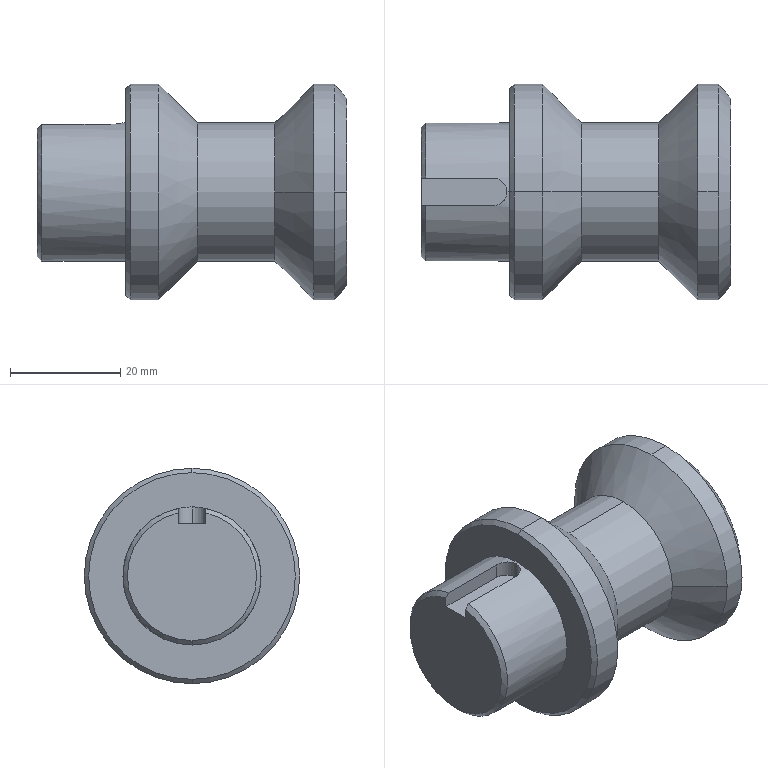Part | SolidWorks | features BaseBody 1 | 1 solid | 28 faces | box 56 x 39 x 39 mm | volume 37628 mm3 | cylinder 12 | cone 10 | plane 6 | commonest cylinder face diameters 25 x4 39 x4 5 x2 34 x2
STEP:
#1=CARTESIAN_POINT('',(61.076,0.,-17.));
#2=VERTEX_POINT('',#1);
#3=CARTESIAN_POINT('',(61.076,-17.,0.));
#4=VERTEX_POINT('',#3);
#5=CARTESIAN_POINT('',(61.076,0.,0.));
#6=DIRECTION('',(-1.,0.,0.));
#7=DIRECTION('',(0.,0.,1.));
#8=AXIS2_PLACEMENT_3D('',#5,#6,#7);
#9=CIRCLE('',#8,17.);
#10=EDGE_CURVE('',#2,#4,#9,.T.);
#11=ORIENTED_EDGE('',*,*,#10,.F.);
#12=CARTESIAN_POINT('',(58.576,0.,-17.));
#13=VERTEX_POINT('',#12);
#14=CARTESIAN_POINT('',(0.,0.,-17.));
#15=DIRECTION('',(-1.,0.,0.));
#16=VECTOR('',#15,1000.);
#17=LINE('',#14,#16);
#18=EDGE_CURVE('',#2,#13,#17,.T.);
#19=ORIENTED_EDGE('',*,*,#18,.T.);
#20=CARTESIAN_POINT('',(58.576,0.,17.));
#21=VERTEX_POINT('',#20);
#22=CARTESIAN_POINT('',(58.576,0.,0.));
#23=DIRECTION('',(1.,0.,0.));
#24=DIRECTION('',(0.,0.,1.));
#25=AXIS2_PLACEMENT_3D('',#22,#23,#24);
#26=CIRCLE('',#25,17.);
#27=EDGE_CURVE('',#21,#13,#26,.T.);
#28=ORIENTED_EDGE('',*,*,#27,.F.);
#29=CARTESIAN_POINT('',(61.076,0.,17.));
#30=VERTEX_POINT('',#29);
#31=CARTESIAN_POINT('',(0.,0.,17.));
#32=DIRECTION('',(-1.,0.,0.));
#33=VECTOR('',#32,1000.);
#34=LINE('',#31,#33);
#35=EDGE_CURVE('',#30,#21,#34,.T.);
#36=ORIENTED_EDGE('',*,*,#35,.F.);
#37=CARTESIAN_POINT('',(61.076,0.,0.));
#38=DIRECTION('',(-1.,0.,0.));
#39=DIRECTION('',(0.,0.,1.));
#40=AXIS2_PLACEMENT_3D('',#37,#38,#39);
#41=CIRCLE('',#40,17.);
#42=EDGE_CURVE('',#4,#30,#41,.T.);
#43=ORIENTED_EDGE('',*,*,#42,.F.);
#44=EDGE_LOOP('',(#11,#19,#28,#36,#43));
#45=FACE_OUTER_BOUND('',#44,.T.);
#46=CARTESIAN_POINT('',(0.,0.,0.));
#47=DIRECTION('',(-1.,0.,0.));
#48=DIRECTION('',(0.,0.,1.));
#49=AXIS2_PLACEMENT_3D('',#46,#47,#48);
#50=CYLINDRICAL_SURFACE('',#49,17.);
#51=ADVANCED_FACE('',(#45),#50,.F.);
#52=ORIENTED_EDGE('',*,*,#42,.T.);
#53=CARTESIAN_POINT('',(61.076,17.,0.));
#54=VERTEX_POINT('',#53);
#55=CARTESIAN_POINT('',(61.076,0.,0.));
#56=DIRECTION('',(-1.,0.,0.));
#57=DIRECTION('',(0.,0.,1.));
#58=AXIS2_PLACEMENT_3D('',#55,#56,#57);
#59=CIRCLE('',#58,17.);
#60=EDGE_CURVE('',#30,#54,#59,.T.);
#61=ORIENTED_EDGE('',*,*,#60,.T.);
#62=CARTESIAN_POINT('',(58.876,19.5,0.));
#63=VERTEX_POINT('',#62);
#64=CARTESIAN_POINT('',(58.876,19.5,0.));
#65=DIRECTION('',(-0.6606,0.7507,0.));
#66=VECTOR('',#65,1000.);
#67=LINE('',#64,#66);
#68=EDGE_CURVE('',#54,#63,#67,.T.);
#69=ORIENTED_EDGE('',*,*,#68,.T.);
#70=CARTESIAN_POINT('',(58.876,0.,19.5));
#71=VERTEX_POINT('',#70);
#72=CARTESIAN_POINT('',(58.876,0.,0.));
#73=DIRECTION('',(1.,0.,0.));
#74=DIRECTION('',(0.,0.,-1.));
#75=AXIS2_PLACEMENT_3D('',#72,#73,#74);
#76=CIRCLE('',#75,19.5);
#77=EDGE_CURVE('',#63,#71,#76,.T.);
#78=ORIENTED_EDGE('',*,*,#77,.T.);
#79=CARTESIAN_POINT('',(58.876,-19.5,0.));
#80=VERTEX_POINT('',#79);
#81=CARTESIAN_POINT('',(58.876,0.,0.));
#82=DIRECTION('',(1.,0.,0.));
#83=DIRECTION('',(0.,0.,-1.));
#84=AXIS2_PLACEMENT_3D('',#81,#82,#83);
#85=CIRCLE('',#84,19.5);
#86=EDGE_CURVE('',#71,#80,#85,.T.);
#87=ORIENTED_EDGE('',*,*,#86,.T.);
#88=CARTESIAN_POINT('',(58.876,-19.5,0.));
#89=DIRECTION('',(-0.6606,-0.7507,0.));
#90=VECTOR('',#89,1000.);
#91=LINE('',#88,#90);
#92=EDGE_CURVE('',#4,#80,#91,.T.);
#93=ORIENTED_EDGE('',*,*,#92,.F.);
#94=EDGE_LOOP('',(#52,#61,#69,#78,#87,#93));
#95=FACE_OUTER_BOUND('',#94,.T.);
#96=CARTESIAN_POINT('',(58.876,0.,0.));
#97=DIRECTION('',(-1.,0.,0.));
#98=DIRECTION('',(0.,-1.,0.));
#99=AXIS2_PLACEMENT_3D('',#96,#97,#98);
#100=CONICAL_SURFACE('',#99,19.5,0.8491);
#101=ADVANCED_FACE('',(#95),#100,.T.);
#102=CARTESIAN_POINT('',(58.876,0.,-19.5));
#103=VERTEX_POINT('',#102);
#104=CARTESIAN_POINT('',(58.876,0.,0.));
#105=DIRECTION('',(1.,0.,0.));
#106=DIRECTION('',(0.,0.,-1.));
#107=AXIS2_PLACEMENT_3D('',#104,#105,#106);
#108=CIRCLE('',#107,19.5);
#109=EDGE_CURVE('',#103,#63,#108,.T.);
#110=ORIENTED_EDGE('',*,*,#109,.F.);
#111=CARTESIAN_POINT('',(55.076,0.,-19.5));
#112=VERTEX_POINT('',#111);
#113=CARTESIAN_POINT('',(0.,0.,-19.5));
#114=DIRECTION('',(-1.,0.,0.));
#115=VECTOR('',#114,1000.);
#116=LINE('',#113,#115);
#117=EDGE_CURVE('',#103,#112,#116,.T.);
#118=ORIENTED_EDGE('',*,*,#117,.T.);
#119=CARTESIAN_POINT('',(55.076,19.5,0.));
#120=VERTEX_POINT('',#119);
#121=CARTESIAN_POINT('',(55.076,0.,0.));
#122=DIRECTION('',(1.,0.,0.));
#123=DIRECTION('',(0.,0.,1.));
#124=AXIS2_PLACEMENT_3D('',#121,#122,#123);
#125=CIRCLE('',#124,19.5);
#126=EDGE_CURVE('',#112,#120,#125,.T.);
#127=ORIENTED_EDGE('',*,*,#126,.T.);
#128=CARTESIAN_POINT('',(55.076,0.,19.5));
#129=VERTEX_POINT('',#128);
#130=CARTESIAN_POINT('',(55.076,0.,0.));
#131=DIRECTION('',(1.,0.,0.));
#132=DIRECTION('',(0.,0.,1.));
#133=AXIS2_PLACEMENT_3D('',#130,#131,#132);
#134=CIRCLE('',#133,19.5);
#135=EDGE_CURVE('',#120,#129,#134,.T.);
#136=ORIENTED_EDGE('',*,*,#135,.T.);
#137=CARTESIAN_POINT('',(0.,0.,19.5));
#138=DIRECTION('',(-1.,0.,0.));
#139=VECTOR('',#138,1000.);
#140=LINE('',#137,#139);
#141=EDGE_CURVE('',#71,#129,#140,.T.);
#142=ORIENTED_EDGE('',*,*,#141,.F.);
#143=ORIENTED_EDGE('',*,*,#77,.F.);
#144=EDGE_LOOP('',(#110,#118,#127,#136,#142,#143));
#145=FACE_OUTER_BOUND('',#144,.T.);
#146=CARTESIAN_POINT('',(0.,0.,0.));
#147=DIRECTION('',(-1.,0.,0.));
#148=DIRECTION('',(0.,0.,1.));
#149=AXIS2_PLACEMENT_3D('',#146,#147,#148);
#150=CYLINDRICAL_SURFACE('',#149,19.5);
#151=ADVANCED_FACE('',(#145),#150,.T.);
#152=CARTESIAN_POINT('',(48.076,0.,12.5));
#153=VERTEX_POINT('',#152);
#154=CARTESIAN_POINT('',(48.076,-12.5,0.));
#155=VERTEX_POINT('',#154);
#156=CARTESIAN_POINT('',(48.076,0.,0.));
#157=DIRECTION('',(1.,0.,0.));
#158=DIRECTION('',(0.,0.,1.));
#159=AXIS2_PLACEMENT_3D('',#156,#157,#158);
#160=CIRCLE('',#159,12.5);
#161=EDGE_CURVE('',#153,#155,#160,.T.);
#162=ORIENTED_EDGE('',*,*,#161,.T.);
#163=CARTESIAN_POINT('',(55.076,-19.5,0.));
#164=VERTEX_POINT('',#163);
#165=CARTESIAN_POINT('',(55.076,-19.5,0.));
#166=DIRECTION('',(0.7071,-0.7071,0.));
#167=VECTOR('',#166,1000.);
#168=LINE('',#165,#167);
#169=EDGE_CURVE('',#155,#164,#168,.T.);
#170=ORIENTED_EDGE('',*,*,#169,.T.);
#171=CARTESIAN_POINT('',(55.076,0.,0.));
#172=DIRECTION('',(1.,0.,0.));
#173=DIRECTION('',(0.,0.,1.));
#174=AXIS2_PLACEMENT_3D('',#171,#172,#173);
#175=CIRCLE('',#174,19.5);
#176=EDGE_CURVE('',#129,#164,#175,.T.);
#177=ORIENTED_EDGE('',*,*,#176,.F.);
#178=ORIENTED_EDGE('',*,*,#135,.F.);
#179=CARTESIAN_POINT('',(48.076,12.5,0.));
#180=VERTEX_POINT('',#179);
#181=CARTESIAN_POINT('',(55.076,19.5,0.));
#182=DIRECTION('',(0.7071,0.7071,0.));
#183=VECTOR('',#182,1000.);
#184=LINE('',#181,#183);
#185=EDGE_CURVE('',#180,#120,#184,.T.);
#186=ORIENTED_EDGE('',*,*,#185,.F.);
#187=CARTESIAN_POINT('',(48.076,0.,0.));
#188=DIRECTION('',(1.,0.,0.));
#189=DIRECTION('',(0.,0.,1.));
#190=AXIS2_PLACEMENT_3D('',#187,#188,#189);
#191=CIRCLE('',#190,12.5);
#192=EDGE_CURVE('',#180,#153,#191,.T.);
#193=ORIENTED_EDGE('',*,*,#192,.T.);
#194=EDGE_LOOP('',(#162,#170,#177,#178,#186,#193));
#195=FACE_OUTER_BOUND('',#194,.T.);
#196=CARTESIAN_POINT('',(55.076,0.,0.));
#197=DIRECTION('',(1.,0.,0.));
#198=DIRECTION('',(0.,1.,0.));
#199=AXIS2_PLACEMENT_3D('',#196,#197,#198);
#200=CONICAL_SURFACE('',#199,19.5,0.7854);
#201=ADVANCED_FACE('',(#195),#200,.T.);
#202=CARTESIAN_POINT('',(48.076,0.,-12.5));
#203=VERTEX_POINT('',#202);
#204=CARTESIAN_POINT('',(48.076,0.,0.));
#205=DIRECTION('',(1.,0.,0.));
#206=DIRECTION('',(0.,0.,1.));
#207=AXIS2_PLACEMENT_3D('',#204,#205,#206);
#208=CIRCLE('',#207,12.5);
#209=EDGE_CURVE('',#203,#180,#208,.T.);
#210=ORIENTED_EDGE('',*,*,#209,.F.);
#211=CARTESIAN_POINT('',(34.076,0.,-12.5));
#212=VERTEX_POINT('',#211);
#213=CARTESIAN_POINT('',(0.,0.,-12.5));
#214=DIRECTION('',(-1.,0.,0.));
#215=VECTOR('',#214,1000.);
#216=LINE('',#213,#215);
#217=EDGE_CURVE('',#203,#212,#216,.T.);
#218=ORIENTED_EDGE('',*,*,#217,.T.);
#219=CARTESIAN_POINT('',(34.076,0.,12.5));
#220=VERTEX_POINT('',#219);
#221=CARTESIAN_POINT('',(34.076,0.,0.));
#222=DIRECTION('',(1.,0.,0.));
#223=DIRECTION('',(0.,0.,1.));
#224=AXIS2_PLACEMENT_3D('',#221,#222,#223);
#225=CIRCLE('',#224,12.5);
#226=EDGE_CURVE('',#212,#220,#225,.T.);
#227=ORIENTED_EDGE('',*,*,#226,.T.);
#228=CARTESIAN_POINT('',(0.,0.,12.5));
#229=DIRECTION('',(-1.,0.,0.));
#230=VECTOR('',#229,1000.);
#231=LINE('',#228,#230);
#232=EDGE_CURVE('',#153,#220,#231,.T.);
#233=ORIENTED_EDGE('',*,*,#232,.F.);
#234=ORIENTED_EDGE('',*,*,#192,.F.);
#235=EDGE_LOOP('',(#210,#218,#227,#233,#234));
#236=FACE_OUTER_BOUND('',#235,.T.);
#237=CARTESIAN_POINT('',(0.,0.,0.));
#238=DIRECTION('',(-1.,0.,0.));
#239=DIRECTION('',(0.,0.,1.));
#240=AXIS2_PLACEMENT_3D('',#237,#238,#239);
#241=CYLINDRICAL_SURFACE('',#240,12.5);
#242=ADVANCED_FACE('',(#236),#241,.T.);
#243=ORIENTED_EDGE('',*,*,#226,.F.);
#244=CARTESIAN_POINT('',(27.076,0.,-19.5));
#245=VERTEX_POINT('',#244);
#246=CARTESIAN_POINT('',(27.076,0.,-19.5));
#247=DIRECTION('',(-0.7071,0.,-0.7071));
#248=VECTOR('',#247,1000.);
#249=LINE('',#246,#248);
#250=EDGE_CURVE('',#212,#245,#249,.T.);
#251=ORIENTED_EDGE('',*,*,#250,.T.);
#252=CARTESIAN_POINT('',(27.076,0.,19.5));
#253=VERTEX_POINT('',#252);
#254=CARTESIAN_POINT('',(27.076,0.,0.));
#255=DIRECTION('',(1.,0.,0.));
#256=DIRECTION('',(0.,0.,-1.));
#257=AXIS2_PLACEMENT_3D('',#254,#255,#256);
#258=CIRCLE('',#257,19.5);
#259=EDGE_CURVE('',#245,#253,#258,.T.);
#260=ORIENTED_EDGE('',*,*,#259,.T.);
#261=CARTESIAN_POINT('',(27.076,0.,19.5));
#262=DIRECTION('',(-0.7071,0.,0.7071));
#263=VECTOR('',#262,1000.);
#264=LINE('',#261,#263);
#265=EDGE_CURVE('',#220,#253,#264,.T.);
#266=ORIENTED_EDGE('',*,*,#265,.F.);
#267=EDGE_LOOP('',(#243,#251,#260,#266));
#268=FACE_OUTER_BOUND('',#267,.T.);
#269=CARTESIAN_POINT('',(27.076,0.,0.));
#270=DIRECTION('',(-1.,0.,0.));
#271=DIRECTION('',(0.,0.,1.));
#272=AXIS2_PLACEMENT_3D('',#269,#270,#271);
#273=CONICAL_SURFACE('',#272,19.5,0.7854);
#274=ADVANCED_FACE('',(#268),#273,.T.);
#275=ORIENTED_EDGE('',*,*,#259,.F.);
#276=CARTESIAN_POINT('',(21.876,0.,-19.5));
#277=VERTEX_POINT('',#276);
#278=CARTESIAN_POINT('',(0.,0.,-19.5));
#279=DIRECTION('',(-1.,0.,0.));
#280=VECTOR('',#279,1000.);
#281=LINE('',#278,#280);
#282=EDGE_CURVE('',#245,#277,#281,.T.);
#283=ORIENTED_EDGE('',*,*,#282,.T.);
#284=CARTESIAN_POINT('',(21.876,0.,19.5));
#285=VERTEX_POINT('',#284);
#286=CARTESIAN_POINT('',(21.876,0.,0.));
#287=DIRECTION('',(1.,0.,0.));
#288=DIRECTION('',(0.,0.,1.));
#289=AXIS2_PLACEMENT_3D('',#286,#287,#288);
#290=CIRCLE('',#289,19.5);
#291=EDGE_CURVE('',#277,#285,#290,.T.);
#292=ORIENTED_EDGE('',*,*,#291,.T.);
#293=CARTESIAN_POINT('',(0.,0.,19.5));
#294=DIRECTION('',(-1.,0.,0.));
#295=VECTOR('',#294,1000.);
#296=LINE('',#293,#295);
#297=EDGE_CURVE('',#253,#285,#296,.T.);
#298=ORIENTED_EDGE('',*,*,#297,.F.);
#299=EDGE_LOOP('',(#275,#283,#292,#298));
#300=FACE_OUTER_BOUND('',#299,.T.);
#301=CARTESIAN_POINT('',(0.,0.,0.));
#302=DIRECTION('',(-1.,0.,0.));
#303=DIRECTION('',(0.,0.,1.));
#304=AXIS2_PLACEMENT_3D('',#301,#302,#303);
#305=CYLINDRICAL_SURFACE('',#304,19.5);
#306=ADVANCED_FACE('',(#300),#305,.T.);
#307=CARTESIAN_POINT('',(21.076,0.,-18.7));
#308=VERTEX_POINT('',#307);
#309=CARTESIAN_POINT('',(21.076,0.,18.7));
#310=VERTEX_POINT('',#309);
#311=CARTESIAN_POINT('',(21.076,0.,0.));
#312=DIRECTION('',(1.,0.,0.));
#313=DIRECTION('',(0.,0.,-1.));
#314=AXIS2_PLACEMENT_3D('',#311,#312,#313);
#315=CIRCLE('',#314,18.7);
#316=EDGE_CURVE('',#308,#310,#315,.T.);
#317=ORIENTED_EDGE('',*,*,#316,.T.);
#318=CARTESIAN_POINT('',(21.876,0.,19.5));
#319=DIRECTION('',(0.7071,0.,0.7071));
#320=VECTOR('',#319,1000.);
#321=LINE('',#318,#320);
#322=EDGE_CURVE('',#310,#285,#321,.T.);
#323=ORIENTED_EDGE('',*,*,#322,.T.);
#324=ORIENTED_EDGE('',*,*,#291,.F.);
#325=CARTESIAN_POINT('',(21.876,0.,-19.5));
#326=DIRECTION('',(0.7071,0.,-0.7071));
#327=VECTOR('',#326,1000.);
#328=LINE('',#325,#327);
#329=EDGE_CURVE('',#308,#277,#328,.T.);
#330=ORIENTED_EDGE('',*,*,#329,.F.);
#331=EDGE_LOOP('',(#317,#323,#324,#330));
#332=FACE_OUTER_BOUND('',#331,.T.);
#333=CARTESIAN_POINT('',(21.876,0.,0.));
#334=DIRECTION('',(1.,0.,0.));
#335=DIRECTION('',(0.,0.,-1.));
#336=AXIS2_PLACEMENT_3D('',#333,#334,#335);
#337=CONICAL_SURFACE('',#336,19.5,0.7854);
#338=ADVANCED_FACE('',(#332),#337,.T.);
#339=CARTESIAN_POINT('',(21.076,0.,-12.5));
#340=VERTEX_POINT('',#339);
#341=CARTESIAN_POINT('',(21.076,0.,12.5));
#342=VERTEX_POINT('',#341);
#343=CARTESIAN_POINT('',(21.076,0.,0.));
#344=DIRECTION('',(1.,0.,0.));
#345=DIRECTION('',(0.,0.,1.));
#346=AXIS2_PLACEMENT_3D('',#343,#344,#345);
#347=CIRCLE('',#346,12.5);
#348=EDGE_CURVE('',#340,#342,#347,.T.);
#349=ORIENTED_EDGE('',*,*,#348,.F.);
#350=CARTESIAN_POINT('',(5.876,0.,-12.5));
#351=VERTEX_POINT('',#350);
#352=CARTESIAN_POINT('',(0.,0.,-12.5));
#353=DIRECTION('',(-1.,0.,0.));
#354=VECTOR('',#353,1000.);
#355=LINE('',#352,#354);
#356=EDGE_CURVE('',#340,#351,#355,.T.);
#357=ORIENTED_EDGE('',*,*,#356,.T.);
#358=CARTESIAN_POINT('',(5.876,2.5,12.247));
#359=VERTEX_POINT('',#358);
#360=CARTESIAN_POINT('',(5.876,0.,0.));
#361=DIRECTION('',(1.,0.,0.));
#362=DIRECTION('',(0.,0.,1.));
#363=AXIS2_PLACEMENT_3D('',#360,#361,#362);
#364=CIRCLE('',#363,12.5);
#365=EDGE_CURVE('',#351,#359,#364,.T.);
#366=ORIENTED_EDGE('',*,*,#365,.T.);
#367=CARTESIAN_POINT('',(18.076,2.5,12.247));
#368=VERTEX_POINT('',#367);
#369=CARTESIAN_POINT('',(0.,2.5,12.247));
#370=DIRECTION('',(1.,0.,0.));
#371=VECTOR('',#370,1000.);
#372=LINE('',#369,#371);
#373=EDGE_CURVE('',#359,#368,#372,.T.);
#374=ORIENTED_EDGE('',*,*,#373,.T.);
#375=CARTESIAN_POINT('',(20.576,0.,12.5));
#376=VERTEX_POINT('',#375);
#377=CARTESIAN_POINT('',(18.076,2.5,12.247));
#378=CARTESIAN_POINT('',(18.241,2.5,12.247));
#379=CARTESIAN_POINT('',(18.404,2.484,12.251));
#380=CARTESIAN_POINT('',(18.724,2.42,12.264));
#381=CARTESIAN_POINT('',(18.883,2.372,12.273));
#382=CARTESIAN_POINT('',(19.185,2.246,12.297));
#383=CARTESIAN_POINT('',(19.328,2.17,12.311));
#384=CARTESIAN_POINT('',(19.6,1.988,12.341));
#385=CARTESIAN_POINT('',(19.728,1.883,12.358));
#386=CARTESIAN_POINT('',(20.073,1.539,12.407));
#387=CARTESIAN_POINT('',(20.259,1.261,12.44));
#388=CARTESIAN_POINT('',(20.509,0.6598,12.486));
#389=CARTESIAN_POINT('',(20.576,0.331,12.5));
#390=CARTESIAN_POINT('',(20.576,0.,12.5));
#391=B_SPLINE_CURVE_WITH_KNOTS('',3,(#377,#378,#379,#380,#381,#382,#383,#384,#385,#386,#387,#388,#389,#390),.UNSPECIFIED.,.F.,.F.,(4,2,2,2,2,2,4),(-0.003915,-0.003426,-0.002936,-0.002447,-0.001958,-0.0009788,0.),.UNSPECIFIED.);
#392=EDGE_CURVE('',#368,#376,#391,.T.);
#393=ORIENTED_EDGE('',*,*,#392,.T.);
#394=CARTESIAN_POINT('',(0.,0.,12.5));
#395=DIRECTION('',(-1.,0.,0.));
#396=VECTOR('',#395,1000.);
#397=LINE('',#394,#396);
#398=EDGE_CURVE('',#342,#376,#397,.T.);
#399=ORIENTED_EDGE('',*,*,#398,.F.);
#400=EDGE_LOOP('',(#349,#357,#366,#374,#393,#399));
#401=FACE_OUTER_BOUND('',#400,.T.);
#402=CARTESIAN_POINT('',(0.,0.,0.));
#403=DIRECTION('',(-1.,0.,0.));
#404=DIRECTION('',(0.,0.,1.));
#405=AXIS2_PLACEMENT_3D('',#402,#403,#404);
#406=CYLINDRICAL_SURFACE('',#405,12.5);
#407=ADVANCED_FACE('',(#401),#406,.T.);
#408=CARTESIAN_POINT('',(5.076,-2.5,11.43));
#409=VERTEX_POINT('',#408);
#410=CARTESIAN_POINT('',(5.076,0.,-11.7));
#411=VERTEX_POINT('',#410);
#412=CARTESIAN_POINT('',(5.076,0.,0.));
#413=DIRECTION('',(1.,0.,0.));
#414=DIRECTION('',(0.,0.,-1.));
#415=AXIS2_PLACEMENT_3D('',#412,#413,#414);
#416=CIRCLE('',#415,11.7);
#417=EDGE_CURVE('',#409,#411,#416,.T.);
#418=ORIENTED_EDGE('',*,*,#417,.T.);
#419=CARTESIAN_POINT('',(5.876,0.,-12.5));
#420=DIRECTION('',(0.7071,0.,-0.7071));
#421=VECTOR('',#420,1000.);
#422=LINE('',#419,#421);
#423=EDGE_CURVE('',#411,#351,#422,.T.);
#424=ORIENTED_EDGE('',*,*,#423,.T.);
#425=CARTESIAN_POINT('',(5.876,-2.5,12.247));
#426=VERTEX_POINT('',#425);
#427=CARTESIAN_POINT('',(5.876,0.,0.));
#428=DIRECTION('',(1.,0.,0.));
#429=DIRECTION('',(0.,0.,1.));
#430=AXIS2_PLACEMENT_3D('',#427,#428,#429);
#431=CIRCLE('',#430,12.5);
#432=EDGE_CURVE('',#426,#351,#431,.T.);
#433=ORIENTED_EDGE('',*,*,#432,.F.);
#434=CARTESIAN_POINT('',(5.876,-2.5,12.247));
#435=CARTESIAN_POINT('',(5.609,-2.5,11.975));
#436=CARTESIAN_POINT('',(5.342,-2.5,11.703));
#437=CARTESIAN_POINT('',(5.076,-2.5,11.43));
#438=B_SPLINE_CURVE_WITH_KNOTS('',3,(#434,#435,#436,#437),.UNSPECIFIED.,.F.,.F.,(4,4),(0.,0.001144),.UNSPECIFIED.);
#439=EDGE_CURVE('',#426,#409,#438,.T.);
#440=ORIENTED_EDGE('',*,*,#439,.T.);
#441=EDGE_LOOP('',(#418,#424,#433,#440));
#442=FACE_OUTER_BOUND('',#441,.T.);
#443=CARTESIAN_POINT('',(5.876,0.,0.));
#444=DIRECTION('',(1.,0.,0.));
#445=DIRECTION('',(0.,0.,-1.));
#446=AXIS2_PLACEMENT_3D('',#443,#444,#445);
#447=CONICAL_SURFACE('',#446,12.5,0.7854);
#448=ADVANCED_FACE('',(#442),#447,.T.);
#449=CARTESIAN_POINT('',(20.576,0.,9.5));
#450=VERTEX_POINT('',#449);
#451=CARTESIAN_POINT('',(18.076,2.5,9.5));
#452=VERTEX_POINT('',#451);
#453=CARTESIAN_POINT('',(18.076,0.,9.5));
#454=DIRECTION('',(0.,0.,1.));
#455=DIRECTION('',(1.,0.,0.));
#456=AXIS2_PLACEMENT_3D('',#453,#454,#455);
#457=CIRCLE('',#456,2.5);
#458=EDGE_CURVE('',#450,#452,#457,.T.);
#459=ORIENTED_EDGE('',*,*,#458,.F.);
#460=CARTESIAN_POINT('',(20.576,0.,9.5));
#461=DIRECTION('',(0.,0.,1.));
#462=VECTOR('',#461,1000.);
#463=LINE('',#460,#462);
#464=EDGE_CURVE('',#450,#376,#463,.T.);
#465=ORIENTED_EDGE('',*,*,#464,.T.);
#466=ORIENTED_EDGE('',*,*,#392,.F.);
#467=CARTESIAN_POINT('',(18.076,2.5,9.5));
#468=DIRECTION('',(0.,0.,1.));
#469=VECTOR('',#468,1000.);
#470=LINE('',#467,#469);
#471=EDGE_CURVE('',#452,#368,#470,.T.);
#472=ORIENTED_EDGE('',*,*,#471,.F.);
#473=EDGE_LOOP('',(#459,#465,#466,#472));
#474=FACE_OUTER_BOUND('',#473,.T.);
#475=CARTESIAN_POINT('',(18.076,0.,9.5));
#476=DIRECTION('',(0.,0.,1.));
#477=DIRECTION('',(1.,0.,0.));
#478=AXIS2_PLACEMENT_3D('',#475,#476,#477);
#479=CYLINDRICAL_SURFACE('',#478,2.5);
#480=ADVANCED_FACE('',(#474),#479,.F.);
#481=ORIENTED_EDGE('',*,*,#27,.T.);
#482=CARTESIAN_POINT('',(58.576,0.,0.));
#483=DIRECTION('',(1.,0.,0.));
#484=DIRECTION('',(0.,0.,1.));
#485=AXIS2_PLACEMENT_3D('',#482,#483,#484);
#486=CIRCLE('',#485,17.);
#487=EDGE_CURVE('',#13,#21,#486,.T.);
#488=ORIENTED_EDGE('',*,*,#487,.T.);
#489=EDGE_LOOP('',(#481,#488));
#490=FACE_OUTER_BOUND('',#489,.T.);
#491=CARTESIAN_POINT('',(58.576,0.,0.));
#492=DIRECTION('',(1.,0.,0.));
#493=DIRECTION('',(0.,0.,-1.));
#494=AXIS2_PLACEMENT_3D('',#491,#492,#493);
#495=PLANE('',#494);
#496=ADVANCED_FACE('',(#490),#495,.T.);
#497=ORIENTED_EDGE('',*,*,#18,.F.);
#498=CARTESIAN_POINT('',(61.076,0.,0.));
#499=DIRECTION('',(-1.,0.,0.));
#500=DIRECTION('',(0.,0.,1.));
#501=AXIS2_PLACEMENT_3D('',#498,#499,#500);
#502=CIRCLE('',#501,17.);
#503=EDGE_CURVE('',#54,#2,#502,.T.);
#504=ORIENTED_EDGE('',*,*,#503,.F.);
#505=ORIENTED_EDGE('',*,*,#60,.F.);
#506=ORIENTED_EDGE('',*,*,#35,.T.);
#507=ORIENTED_EDGE('',*,*,#487,.F.);
#508=EDGE_LOOP('',(#497,#504,#505,#506,#507));
#509=FACE_OUTER_BOUND('',#508,.T.);
#510=CARTESIAN_POINT('',(0.,0.,0.));
#511=DIRECTION('',(-1.,0.,0.));
#512=DIRECTION('',(0.,0.,1.));
#513=AXIS2_PLACEMENT_3D('',#510,#511,#512);
#514=CYLINDRICAL_SURFACE('',#513,17.);
#515=ADVANCED_FACE('',(#509),#514,.F.);
#516=ORIENTED_EDGE('',*,*,#68,.F.);
#517=ORIENTED_EDGE('',*,*,#503,.T.);
#518=ORIENTED_EDGE('',*,*,#10,.T.);
#519=ORIENTED_EDGE('',*,*,#92,.T.);
#520=CARTESIAN_POINT('',(58.876,0.,0.));
#521=DIRECTION('',(1.,0.,0.));
#522=DIRECTION('',(0.,0.,-1.));
#523=AXIS2_PLACEMENT_3D('',#520,#521,#522);
#524=CIRCLE('',#523,19.5);
#525=EDGE_CURVE('',#80,#103,#524,.T.);
#526=ORIENTED_EDGE('',*,*,#525,.T.);
#527=ORIENTED_EDGE('',*,*,#109,.T.);
#528=EDGE_LOOP('',(#516,#517,#518,#519,#526,#527));
#529=FACE_OUTER_BOUND('',#528,.T.);
#530=CARTESIAN_POINT('',(58.876,0.,0.));
#531=DIRECTION('',(-1.,0.,0.));
#532=DIRECTION('',(0.,-1.,0.));
#533=AXIS2_PLACEMENT_3D('',#530,#531,#532);
#534=CONICAL_SURFACE('',#533,19.5,0.8491);
#535=ADVANCED_FACE('',(#529),#534,.T.);
#536=ORIENTED_EDGE('',*,*,#117,.F.);
#537=ORIENTED_EDGE('',*,*,#525,.F.);
#538=ORIENTED_EDGE('',*,*,#86,.F.);
#539=ORIENTED_EDGE('',*,*,#141,.T.);
#540=ORIENTED_EDGE('',*,*,#176,.T.);
#541=CARTESIAN_POINT('',(55.076,0.,0.));
#542=DIRECTION('',(1.,0.,0.));
#543=DIRECTION('',(0.,0.,1.));
#544=AXIS2_PLACEMENT_3D('',#541,#542,#543);
#545=CIRCLE('',#544,19.5);
#546=EDGE_CURVE('',#164,#112,#545,.T.);
#547=ORIENTED_EDGE('',*,*,#546,.T.);
#548=EDGE_LOOP('',(#536,#537,#538,#539,#540,#547));
#549=FACE_OUTER_BOUND('',#548,.T.);
#550=CARTESIAN_POINT('',(0.,0.,0.));
#551=DIRECTION('',(-1.,0.,0.));
#552=DIRECTION('',(0.,0.,1.));
#553=AXIS2_PLACEMENT_3D('',#550,#551,#552);
#554=CYLINDRICAL_SURFACE('',#553,19.5);
#555=ADVANCED_FACE('',(#549),#554,.T.);
#556=ORIENTED_EDGE('',*,*,#169,.F.);
#557=CARTESIAN_POINT('',(48.076,0.,0.));
#558=DIRECTION('',(1.,0.,0.));
#559=DIRECTION('',(0.,0.,1.));
#560=AXIS2_PLACEMENT_3D('',#557,#558,#559);
#561=CIRCLE('',#560,12.5);
#562=EDGE_CURVE('',#155,#203,#561,.T.);
#563=ORIENTED_EDGE('',*,*,#562,.T.);
#564=ORIENTED_EDGE('',*,*,#209,.T.);
#565=ORIENTED_EDGE('',*,*,#185,.T.);
#566=ORIENTED_EDGE('',*,*,#126,.F.);
#567=ORIENTED_EDGE('',*,*,#546,.F.);
#568=EDGE_LOOP('',(#556,#563,#564,#565,#566,#567));
#569=FACE_OUTER_BOUND('',#568,.T.);
#570=CARTESIAN_POINT('',(55.076,0.,0.));
#571=DIRECTION('',(1.,0.,0.));
#572=DIRECTION('',(0.,1.,0.));
#573=AXIS2_PLACEMENT_3D('',#570,#571,#572);
#574=CONICAL_SURFACE('',#573,19.5,0.7854);
#575=ADVANCED_FACE('',(#569),#574,.T.);
#576=ORIENTED_EDGE('',*,*,#217,.F.);
#577=ORIENTED_EDGE('',*,*,#562,.F.);
#578=ORIENTED_EDGE('',*,*,#161,.F.);
#579=ORIENTED_EDGE('',*,*,#232,.T.);
#580=CARTESIAN_POINT('',(34.076,0.,0.));
#581=DIRECTION('',(1.,0.,0.));
#582=DIRECTION('',(0.,0.,1.));
#583=AXIS2_PLACEMENT_3D('',#580,#581,#582);
#584=CIRCLE('',#583,12.5);
#585=EDGE_CURVE('',#220,#212,#584,.T.);
#586=ORIENTED_EDGE('',*,*,#585,.T.);
#587=EDGE_LOOP('',(#576,#577,#578,#579,#586));
#588=FACE_OUTER_BOUND('',#587,.T.);
#589=CARTESIAN_POINT('',(0.,0.,0.));
#590=DIRECTION('',(-1.,0.,0.));
#591=DIRECTION('',(0.,0.,1.));
#592=AXIS2_PLACEMENT_3D('',#589,#590,#591);
#593=CYLINDRICAL_SURFACE('',#592,12.5);
#594=ADVANCED_FACE('',(#588),#593,.T.);
#595=ORIENTED_EDGE('',*,*,#250,.F.);
#596=ORIENTED_EDGE('',*,*,#585,.F.);
#597=ORIENTED_EDGE('',*,*,#265,.T.);
#598=CARTESIAN_POINT('',(27.076,0.,0.));
#599=DIRECTION('',(1.,0.,0.));
#600=DIRECTION('',(0.,0.,-1.));
#601=AXIS2_PLACEMENT_3D('',#598,#599,#600);
#602=CIRCLE('',#601,19.5);
#603=EDGE_CURVE('',#253,#245,#602,.T.);
#604=ORIENTED_EDGE('',*,*,#603,.T.);
#605=EDGE_LOOP('',(#595,#596,#597,#604));
#606=FACE_OUTER_BOUND('',#605,.T.);
#607=CARTESIAN_POINT('',(27.076,0.,0.));
#608=DIRECTION('',(-1.,0.,0.));
#609=DIRECTION('',(0.,0.,1.));
#610=AXIS2_PLACEMENT_3D('',#607,#608,#609);
#611=CONICAL_SURFACE('',#610,19.5,0.7854);
#612=ADVANCED_FACE('',(#606),#611,.T.);
#613=ORIENTED_EDGE('',*,*,#282,.F.);
#614=ORIENTED_EDGE('',*,*,#603,.F.);
#615=ORIENTED_EDGE('',*,*,#297,.T.);
#616=CARTESIAN_POINT('',(21.876,0.,0.));
#617=DIRECTION('',(1.,0.,0.));
#618=DIRECTION('',(0.,0.,1.));
#619=AXIS2_PLACEMENT_3D('',#616,#617,#618);
#620=CIRCLE('',#619,19.5);
#621=EDGE_CURVE('',#285,#277,#620,.T.);
#622=ORIENTED_EDGE('',*,*,#621,.T.);
#623=EDGE_LOOP('',(#613,#614,#615,#622));
#624=FACE_OUTER_BOUND('',#623,.T.);
#625=CARTESIAN_POINT('',(0.,0.,0.));
#626=DIRECTION('',(-1.,0.,0.));
#627=DIRECTION('',(0.,0.,1.));
#628=AXIS2_PLACEMENT_3D('',#625,#626,#627);
#629=CYLINDRICAL_SURFACE('',#628,19.5);
#630=ADVANCED_FACE('',(#624),#629,.T.);
#631=ORIENTED_EDGE('',*,*,#322,.F.);
#632=CARTESIAN_POINT('',(21.076,0.,0.));
#633=DIRECTION('',(1.,0.,0.));
#634=DIRECTION('',(0.,0.,-1.));
#635=AXIS2_PLACEMENT_3D('',#632,#633,#634);
#636=CIRCLE('',#635,18.7);
#637=EDGE_CURVE('',#310,#308,#636,.T.);
#638=ORIENTED_EDGE('',*,*,#637,.T.);
#639=ORIENTED_EDGE('',*,*,#329,.T.);
#640=ORIENTED_EDGE('',*,*,#621,.F.);
#641=EDGE_LOOP('',(#631,#638,#639,#640));
#642=FACE_OUTER_BOUND('',#641,.T.);
#643=CARTESIAN_POINT('',(21.876,0.,0.));
#644=DIRECTION('',(1.,0.,0.));
#645=DIRECTION('',(0.,0.,-1.));
#646=AXIS2_PLACEMENT_3D('',#643,#644,#645);
#647=CONICAL_SURFACE('',#646,19.5,0.7854);
#648=ADVANCED_FACE('',(#642),#647,.T.);
#649=CARTESIAN_POINT('',(21.076,0.,0.));
#650=DIRECTION('',(1.,0.,0.));
#651=DIRECTION('',(0.,0.,1.));
#652=AXIS2_PLACEMENT_3D('',#649,#650,#651);
#653=CIRCLE('',#652,12.5);
#654=EDGE_CURVE('',#342,#340,#653,.T.);
#655=ORIENTED_EDGE('',*,*,#654,.T.);
#656=ORIENTED_EDGE('',*,*,#348,.T.);
#657=EDGE_LOOP('',(#655,#656));
#658=FACE_BOUND('',#657,.T.);
#659=ORIENTED_EDGE('',*,*,#316,.F.);
#660=ORIENTED_EDGE('',*,*,#637,.F.);
#661=EDGE_LOOP('',(#659,#660));
#662=FACE_OUTER_BOUND('',#661,.T.);
#663=CARTESIAN_POINT('',(21.076,0.,0.));
#664=DIRECTION('',(-1.,0.,0.));
#665=DIRECTION('',(0.,0.,1.));
#666=AXIS2_PLACEMENT_3D('',#663,#664,#665);
#667=PLANE('',#666);
#668=ADVANCED_FACE('',(#658,#662),#667,.T.);
#669=ORIENTED_EDGE('',*,*,#356,.F.);
#670=ORIENTED_EDGE('',*,*,#654,.F.);
#671=ORIENTED_EDGE('',*,*,#398,.T.);
#672=CARTESIAN_POINT('',(18.076,-2.5,12.247));
#673=VERTEX_POINT('',#672);
#674=CARTESIAN_POINT('',(20.576,0.,12.5));
#675=CARTESIAN_POINT('',(20.576,-0.1655,12.5));
#676=CARTESIAN_POINT('',(20.559,-0.3282,12.497));
#677=CARTESIAN_POINT('',(20.496,-0.6481,12.484));
#678=CARTESIAN_POINT('',(20.447,-0.807,12.475));
#679=CARTESIAN_POINT('',(20.322,-1.109,12.452));
#680=CARTESIAN_POINT('',(20.245,-1.253,12.438));
#681=CARTESIAN_POINT('',(20.064,-1.524,12.407));
#682=CARTESIAN_POINT('',(19.959,-1.652,12.391));
#683=CARTESIAN_POINT('',(19.614,-1.997,12.342));
#684=CARTESIAN_POINT('',(19.336,-2.183,12.309));
#685=CARTESIAN_POINT('',(18.735,-2.433,12.262));
#686=CARTESIAN_POINT('',(18.407,-2.5,12.247));
#687=CARTESIAN_POINT('',(18.076,-2.5,12.247));
#688=B_SPLINE_CURVE_WITH_KNOTS('',3,(#674,#675,#676,#677,#678,#679,#680,#681,#682,#683,#684,#685,#686,#687),.UNSPECIFIED.,.F.,.F.,(4,2,2,2,2,2,4),(0.,0.0004894,0.0009788,0.001468,0.001958,0.002936,0.003915),.UNSPECIFIED.);
#689=EDGE_CURVE('',#376,#673,#688,.T.);
#690=ORIENTED_EDGE('',*,*,#689,.T.);
#691=CARTESIAN_POINT('',(0.,-2.5,12.247));
#692=DIRECTION('',(-1.,0.,0.));
#693=VECTOR('',#692,1000.);
#694=LINE('',#691,#693);
#695=EDGE_CURVE('',#673,#426,#694,.T.);
#696=ORIENTED_EDGE('',*,*,#695,.T.);
#697=ORIENTED_EDGE('',*,*,#432,.T.);
#698=EDGE_LOOP('',(#669,#670,#671,#690,#696,#697));
#699=FACE_OUTER_BOUND('',#698,.T.);
#700=CARTESIAN_POINT('',(0.,0.,0.));
#701=DIRECTION('',(-1.,0.,0.));
#702=DIRECTION('',(0.,0.,1.));
#703=AXIS2_PLACEMENT_3D('',#700,#701,#702);
#704=CYLINDRICAL_SURFACE('',#703,12.5);
#705=ADVANCED_FACE('',(#699),#704,.T.);
#706=ORIENTED_EDGE('',*,*,#423,.F.);
#707=CARTESIAN_POINT('',(5.076,2.5,11.43));
#708=VERTEX_POINT('',#707);
#709=CARTESIAN_POINT('',(5.076,0.,0.));
#710=DIRECTION('',(1.,0.,0.));
#711=DIRECTION('',(0.,0.,-1.));
#712=AXIS2_PLACEMENT_3D('',#709,#710,#711);
#713=CIRCLE('',#712,11.7);
#714=EDGE_CURVE('',#411,#708,#713,.T.);
#715=ORIENTED_EDGE('',*,*,#714,.T.);
#716=CARTESIAN_POINT('',(5.076,2.5,11.43));
#717=CARTESIAN_POINT('',(5.342,2.5,11.703));
#718=CARTESIAN_POINT('',(5.609,2.5,11.975));
#719=CARTESIAN_POINT('',(5.876,2.5,12.247));
#720=B_SPLINE_CURVE_WITH_KNOTS('',3,(#716,#717,#718,#719),.UNSPECIFIED.,.F.,.F.,(4,4),(0.,0.001144),.UNSPECIFIED.);
#721=EDGE_CURVE('',#708,#359,#720,.T.);
#722=ORIENTED_EDGE('',*,*,#721,.T.);
#723=ORIENTED_EDGE('',*,*,#365,.F.);
#724=EDGE_LOOP('',(#706,#715,#722,#723));
#725=FACE_OUTER_BOUND('',#724,.T.);
#726=CARTESIAN_POINT('',(5.876,0.,0.));
#727=DIRECTION('',(1.,0.,0.));
#728=DIRECTION('',(0.,0.,-1.));
#729=AXIS2_PLACEMENT_3D('',#726,#727,#728);
#730=CONICAL_SURFACE('',#729,12.5,0.7854);
#731=ADVANCED_FACE('',(#725),#730,.T.);
#732=CARTESIAN_POINT('',(18.076,-2.5,9.5));
#733=VERTEX_POINT('',#732);
#734=CARTESIAN_POINT('',(18.076,-2.5,9.5));
#735=DIRECTION('',(0.,0.,1.));
#736=VECTOR('',#735,1000.);
#737=LINE('',#734,#736);
#738=EDGE_CURVE('',#733,#673,#737,.T.);
#739=ORIENTED_EDGE('',*,*,#738,.F.);
#740=CARTESIAN_POINT('',(5.076,-2.5,9.5));
#741=VERTEX_POINT('',#740);
#742=CARTESIAN_POINT('',(-6.324,-2.5,9.5));
#743=DIRECTION('',(1.,0.,0.));
#744=VECTOR('',#743,1000.);
#745=LINE('',#742,#744);
#746=EDGE_CURVE('',#741,#733,#745,.T.);
#747=ORIENTED_EDGE('',*,*,#746,.F.);
#748=CARTESIAN_POINT('',(5.076,-2.5,9.5));
#749=DIRECTION('',(0.,0.,-1.));
#750=VECTOR('',#749,1000.);
#751=LINE('',#748,#750);
#752=EDGE_CURVE('',#409,#741,#751,.T.);
#753=ORIENTED_EDGE('',*,*,#752,.F.);
#754=ORIENTED_EDGE('',*,*,#439,.F.);
#755=ORIENTED_EDGE('',*,*,#695,.F.);
#756=EDGE_LOOP('',(#739,#747,#753,#754,#755));
#757=FACE_OUTER_BOUND('',#756,.T.);
#758=CARTESIAN_POINT('',(-6.324,-2.5,9.5));
#759=DIRECTION('',(0.,-1.,0.));
#760=DIRECTION('',(1.,0.,0.));
#761=AXIS2_PLACEMENT_3D('',#758,#759,#760);
#762=PLANE('',#761);
#763=ADVANCED_FACE('',(#757),#762,.F.);
#764=ORIENTED_EDGE('',*,*,#464,.F.);
#765=CARTESIAN_POINT('',(18.076,0.,9.5));
#766=DIRECTION('',(0.,0.,1.));
#767=DIRECTION('',(1.,0.,0.));
#768=AXIS2_PLACEMENT_3D('',#765,#766,#767);
#769=CIRCLE('',#768,2.5);
#770=EDGE_CURVE('',#733,#450,#769,.T.);
#771=ORIENTED_EDGE('',*,*,#770,.F.);
#772=ORIENTED_EDGE('',*,*,#738,.T.);
#773=ORIENTED_EDGE('',*,*,#689,.F.);
#774=EDGE_LOOP('',(#764,#771,#772,#773));
#775=FACE_OUTER_BOUND('',#774,.T.);
#776=CARTESIAN_POINT('',(18.076,0.,9.5));
#777=DIRECTION('',(0.,0.,1.));
#778=DIRECTION('',(1.,0.,0.));
#779=AXIS2_PLACEMENT_3D('',#776,#777,#778);
#780=CYLINDRICAL_SURFACE('',#779,2.5);
#781=ADVANCED_FACE('',(#775),#780,.F.);
#782=ORIENTED_EDGE('',*,*,#721,.F.);
#783=CARTESIAN_POINT('',(5.076,2.5,9.5));
#784=VERTEX_POINT('',#783);
#785=CARTESIAN_POINT('',(5.076,2.5,9.5));
#786=DIRECTION('',(0.,0.,1.));
#787=VECTOR('',#786,1000.);
#788=LINE('',#785,#787);
#789=EDGE_CURVE('',#784,#708,#788,.T.);
#790=ORIENTED_EDGE('',*,*,#789,.F.);
#791=CARTESIAN_POINT('',(-6.324,2.5,9.5));
#792=DIRECTION('',(-1.,0.,0.));
#793=VECTOR('',#792,1000.);
#794=LINE('',#791,#793);
#795=EDGE_CURVE('',#452,#784,#794,.T.);
#796=ORIENTED_EDGE('',*,*,#795,.F.);
#797=ORIENTED_EDGE('',*,*,#471,.T.);
#798=ORIENTED_EDGE('',*,*,#373,.F.);
#799=EDGE_LOOP('',(#782,#790,#796,#797,#798));
#800=FACE_OUTER_BOUND('',#799,.T.);
#801=CARTESIAN_POINT('',(-6.324,2.5,9.5));
#802=DIRECTION('',(0.,1.,0.));
#803=DIRECTION('',(0.,0.,1.));
#804=AXIS2_PLACEMENT_3D('',#801,#802,#803);
#805=PLANE('',#804);
#806=ADVANCED_FACE('',(#800),#805,.F.);
#807=ORIENTED_EDGE('',*,*,#789,.T.);
#808=ORIENTED_EDGE('',*,*,#714,.F.);
#809=ORIENTED_EDGE('',*,*,#417,.F.);
#810=ORIENTED_EDGE('',*,*,#752,.T.);
#811=CARTESIAN_POINT('',(5.076,0.,9.5));
#812=DIRECTION('',(0.,1.,0.));
#813=VECTOR('',#812,1000.);
#814=LINE('',#811,#813);
#815=EDGE_CURVE('',#741,#784,#814,.T.);
#816=ORIENTED_EDGE('',*,*,#815,.T.);
#817=EDGE_LOOP('',(#807,#808,#809,#810,#816));
#818=FACE_OUTER_BOUND('',#817,.T.);
#819=CARTESIAN_POINT('',(5.076,0.,0.));
#820=DIRECTION('',(-1.,0.,0.));
#821=DIRECTION('',(0.,0.,1.));
#822=AXIS2_PLACEMENT_3D('',#819,#820,#821);
#823=PLANE('',#822);
#824=ADVANCED_FACE('',(#818),#823,.T.);
#825=ORIENTED_EDGE('',*,*,#795,.T.);
#826=ORIENTED_EDGE('',*,*,#815,.F.);
#827=ORIENTED_EDGE('',*,*,#746,.T.);
#828=ORIENTED_EDGE('',*,*,#770,.T.);
#829=ORIENTED_EDGE('',*,*,#458,.T.);
#830=EDGE_LOOP('',(#825,#826,#827,#828,#829));
#831=FACE_OUTER_BOUND('',#830,.T.);
#832=CARTESIAN_POINT('',(18.076,0.,9.5));
#833=DIRECTION('',(0.,0.,1.));
#834=DIRECTION('',(1.,0.,0.));
#835=AXIS2_PLACEMENT_3D('',#832,#833,#834);
#836=PLANE('',#835);
#837=ADVANCED_FACE('',(#831),#836,.T.);
#838=CLOSED_SHELL('',(#51,#101,#151,#201,#242,#274,#306,#338,#407,#448,#480,#496,#515,#535,#555,#575,#594,#612,#630,#648,#668,#705,#731,#763,#781,#806,#824,#837));
#839=MANIFOLD_SOLID_BREP('',#838);
#840=CARTESIAN_POINT('',(0.,0.,0.));
#841=DIRECTION('',(0.,0.,1.));
#842=DIRECTION('',(1.,0.,0.));
#843=AXIS2_PLACEMENT_3D('',#840,#841,#842);
#844=(LENGTH_UNIT()NAMED_UNIT(*)SI_UNIT(.MILLI.,.METRE.));
#845=UNCERTAINTY_MEASURE_WITH_UNIT(LENGTH_MEASURE(0.00001),#844,'','');
#846=(NAMED_UNIT(*)PLANE_ANGLE_UNIT()SI_UNIT($,.RADIAN.));
#847=(NAMED_UNIT(*)SI_UNIT($,.STERADIAN.)SOLID_ANGLE_UNIT());
#848=(GEOMETRIC_REPRESENTATION_CONTEXT(3)GLOBAL_UNCERTAINTY_ASSIGNED_CONTEXT((#845))GLOBAL_UNIT_ASSIGNED_CONTEXT((#844,#846,#847))REPRESENTATION_CONTEXT('',''));
#849=ADVANCED_BREP_SHAPE_REPRESENTATION('',(#839,#843),#848);